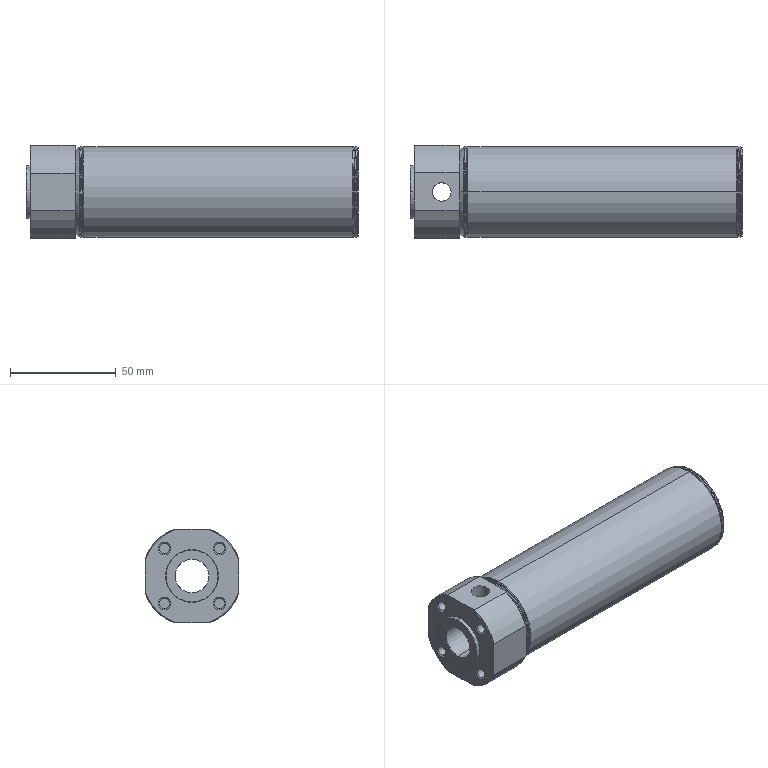Part | SolidWorks | features HoleWzd 2, BaseBody 1, ICE 1 | 1 solid | 91 faces | box 157 x 44 x 44 mm | volume 70964 mm3 | cone 34 | cylinder 30 | plane 15 | spline 12 | commonest cylinder face diameters 4.917 x8 8.8 x4 47.5 x4 3 x2 8.566 x2 16 x2